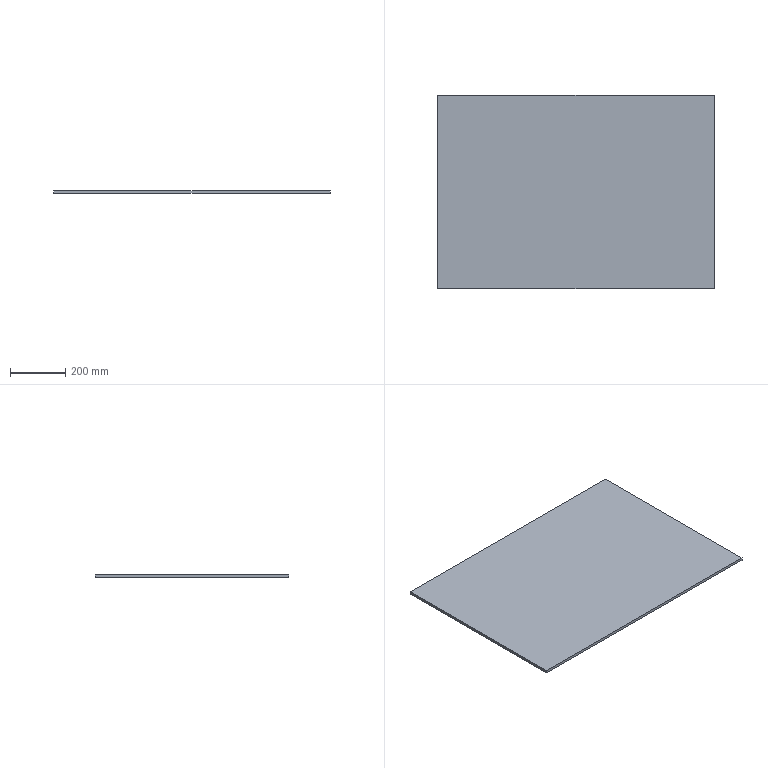Part | SolidWorks | features Extrusion 1 | 1 solid | 6 faces | box 1000 x 700 x 10 mm | volume 7000000 mm3 | plane 6
STEP:
#1=CARTESIAN_POINT('',(500.,-350.,0.));
#2=VERTEX_POINT('',#1);
#3=CARTESIAN_POINT('',(500.,350.,0.));
#4=VERTEX_POINT('',#3);
#5=CARTESIAN_POINT('',(500.,350.,0.));
#6=DIRECTION('',(0.,1.,0.));
#7=VECTOR('',#6,1000.);
#8=LINE('',#5,#7);
#9=EDGE_CURVE('',#2,#4,#8,.T.);
#10=ORIENTED_EDGE('',*,*,#9,.T.);
#11=CARTESIAN_POINT('',(500.,350.,10.));
#12=VERTEX_POINT('',#11);
#13=CARTESIAN_POINT('',(500.,350.,10.));
#14=DIRECTION('',(0.,0.,-1.));
#15=VECTOR('',#14,1000.);
#16=LINE('',#13,#15);
#17=EDGE_CURVE('',#12,#4,#16,.T.);
#18=ORIENTED_EDGE('',*,*,#17,.F.);
#19=CARTESIAN_POINT('',(500.,-350.,10.));
#20=VERTEX_POINT('',#19);
#21=CARTESIAN_POINT('',(500.,350.,10.));
#22=DIRECTION('',(0.,1.,0.));
#23=VECTOR('',#22,1000.);
#24=LINE('',#21,#23);
#25=EDGE_CURVE('',#20,#12,#24,.T.);
#26=ORIENTED_EDGE('',*,*,#25,.F.);
#27=CARTESIAN_POINT('',(500.,-350.,10.));
#28=DIRECTION('',(0.,0.,-1.));
#29=VECTOR('',#28,1000.);
#30=LINE('',#27,#29);
#31=EDGE_CURVE('',#20,#2,#30,.T.);
#32=ORIENTED_EDGE('',*,*,#31,.T.);
#33=EDGE_LOOP('',(#10,#18,#26,#32));
#34=FACE_OUTER_BOUND('',#33,.T.);
#35=CARTESIAN_POINT('',(500.,350.,10.));
#36=DIRECTION('',(-1.,0.,0.));
#37=DIRECTION('',(0.,-1.,0.));
#38=AXIS2_PLACEMENT_3D('',#35,#36,#37);
#39=PLANE('',#38);
#40=ADVANCED_FACE('',(#34),#39,.F.);
#41=CARTESIAN_POINT('',(-500.,350.,0.));
#42=VERTEX_POINT('',#41);
#43=CARTESIAN_POINT('',(-500.,350.,0.));
#44=DIRECTION('',(-1.,0.,0.));
#45=VECTOR('',#44,1000.);
#46=LINE('',#43,#45);
#47=EDGE_CURVE('',#4,#42,#46,.T.);
#48=ORIENTED_EDGE('',*,*,#47,.T.);
#49=CARTESIAN_POINT('',(-500.,350.,10.));
#50=VERTEX_POINT('',#49);
#51=CARTESIAN_POINT('',(-500.,350.,10.));
#52=DIRECTION('',(0.,0.,-1.));
#53=VECTOR('',#52,1000.);
#54=LINE('',#51,#53);
#55=EDGE_CURVE('',#50,#42,#54,.T.);
#56=ORIENTED_EDGE('',*,*,#55,.F.);
#57=CARTESIAN_POINT('',(-500.,350.,10.));
#58=DIRECTION('',(-1.,0.,0.));
#59=VECTOR('',#58,1000.);
#60=LINE('',#57,#59);
#61=EDGE_CURVE('',#12,#50,#60,.T.);
#62=ORIENTED_EDGE('',*,*,#61,.F.);
#63=ORIENTED_EDGE('',*,*,#17,.T.);
#64=EDGE_LOOP('',(#48,#56,#62,#63));
#65=FACE_OUTER_BOUND('',#64,.T.);
#66=CARTESIAN_POINT('',(-500.,350.,10.));
#67=DIRECTION('',(0.,-1.,0.));
#68=DIRECTION('',(0.,0.,-1.));
#69=AXIS2_PLACEMENT_3D('',#66,#67,#68);
#70=PLANE('',#69);
#71=ADVANCED_FACE('',(#65),#70,.F.);
#72=CARTESIAN_POINT('',(-500.,-350.,0.));
#73=VERTEX_POINT('',#72);
#74=CARTESIAN_POINT('',(-500.,350.,0.));
#75=DIRECTION('',(0.,-1.,0.));
#76=VECTOR('',#75,1000.);
#77=LINE('',#74,#76);
#78=EDGE_CURVE('',#42,#73,#77,.T.);
#79=ORIENTED_EDGE('',*,*,#78,.T.);
#80=CARTESIAN_POINT('',(-500.,-350.,10.));
#81=VERTEX_POINT('',#80);
#82=CARTESIAN_POINT('',(-500.,-350.,10.));
#83=DIRECTION('',(0.,0.,-1.));
#84=VECTOR('',#83,1000.);
#85=LINE('',#82,#84);
#86=EDGE_CURVE('',#81,#73,#85,.T.);
#87=ORIENTED_EDGE('',*,*,#86,.F.);
#88=CARTESIAN_POINT('',(-500.,350.,10.));
#89=DIRECTION('',(0.,-1.,0.));
#90=VECTOR('',#89,1000.);
#91=LINE('',#88,#90);
#92=EDGE_CURVE('',#50,#81,#91,.T.);
#93=ORIENTED_EDGE('',*,*,#92,.F.);
#94=ORIENTED_EDGE('',*,*,#55,.T.);
#95=EDGE_LOOP('',(#79,#87,#93,#94));
#96=FACE_OUTER_BOUND('',#95,.T.);
#97=CARTESIAN_POINT('',(-500.,350.,10.));
#98=DIRECTION('',(1.,0.,0.));
#99=DIRECTION('',(0.,1.,0.));
#100=AXIS2_PLACEMENT_3D('',#97,#98,#99);
#101=PLANE('',#100);
#102=ADVANCED_FACE('',(#96),#101,.F.);
#103=CARTESIAN_POINT('',(-500.,-350.,0.));
#104=DIRECTION('',(1.,0.,0.));
#105=VECTOR('',#104,1000.);
#106=LINE('',#103,#105);
#107=EDGE_CURVE('',#73,#2,#106,.T.);
#108=ORIENTED_EDGE('',*,*,#107,.T.);
#109=ORIENTED_EDGE('',*,*,#31,.F.);
#110=CARTESIAN_POINT('',(-500.,-350.,10.));
#111=DIRECTION('',(1.,0.,0.));
#112=VECTOR('',#111,1000.);
#113=LINE('',#110,#112);
#114=EDGE_CURVE('',#81,#20,#113,.T.);
#115=ORIENTED_EDGE('',*,*,#114,.F.);
#116=ORIENTED_EDGE('',*,*,#86,.T.);
#117=EDGE_LOOP('',(#108,#109,#115,#116));
#118=FACE_OUTER_BOUND('',#117,.T.);
#119=CARTESIAN_POINT('',(-500.,-350.,10.));
#120=DIRECTION('',(0.,1.,0.));
#121=DIRECTION('',(0.,0.,1.));
#122=AXIS2_PLACEMENT_3D('',#119,#120,#121);
#123=PLANE('',#122);
#124=ADVANCED_FACE('',(#118),#123,.F.);
#125=ORIENTED_EDGE('',*,*,#25,.T.);
#126=ORIENTED_EDGE('',*,*,#61,.T.);
#127=ORIENTED_EDGE('',*,*,#92,.T.);
#128=ORIENTED_EDGE('',*,*,#114,.T.);
#129=EDGE_LOOP('',(#125,#126,#127,#128));
#130=FACE_OUTER_BOUND('',#129,.T.);
#131=CARTESIAN_POINT('',(0.,0.,10.));
#132=DIRECTION('',(0.,0.,1.));
#133=DIRECTION('',(1.,0.,0.));
#134=AXIS2_PLACEMENT_3D('',#131,#132,#133);
#135=PLANE('',#134);
#136=ADVANCED_FACE('',(#130),#135,.T.);
#137=ORIENTED_EDGE('',*,*,#9,.F.);
#138=ORIENTED_EDGE('',*,*,#107,.F.);
#139=ORIENTED_EDGE('',*,*,#78,.F.);
#140=ORIENTED_EDGE('',*,*,#47,.F.);
#141=EDGE_LOOP('',(#137,#138,#139,#140));
#142=FACE_OUTER_BOUND('',#141,.T.);
#143=CARTESIAN_POINT('',(0.,0.,0.));
#144=DIRECTION('',(0.,0.,1.));
#145=DIRECTION('',(1.,0.,0.));
#146=AXIS2_PLACEMENT_3D('',#143,#144,#145);
#147=PLANE('',#146);
#148=ADVANCED_FACE('',(#142),#147,.F.);
#149=CLOSED_SHELL('',(#40,#71,#102,#124,#136,#148));
#150=MANIFOLD_SOLID_BREP('',#149);
#151=CARTESIAN_POINT('',(0.,0.,0.));
#152=DIRECTION('',(0.,0.,1.));
#153=DIRECTION('',(1.,0.,0.));
#154=AXIS2_PLACEMENT_3D('',#151,#152,#153);
#155=(LENGTH_UNIT()NAMED_UNIT(*)SI_UNIT(.MILLI.,.METRE.));
#156=UNCERTAINTY_MEASURE_WITH_UNIT(LENGTH_MEASURE(0.00001),#155,'','');
#157=(NAMED_UNIT(*)PLANE_ANGLE_UNIT()SI_UNIT($,.RADIAN.));
#158=(NAMED_UNIT(*)SI_UNIT($,.STERADIAN.)SOLID_ANGLE_UNIT());
#159=(GEOMETRIC_REPRESENTATION_CONTEXT(3)GLOBAL_UNCERTAINTY_ASSIGNED_CONTEXT((#156))GLOBAL_UNIT_ASSIGNED_CONTEXT((#155,#157,#158))REPRESENTATION_CONTEXT('',''));
#160=ADVANCED_BREP_SHAPE_REPRESENTATION('',(#150,#154),#159);